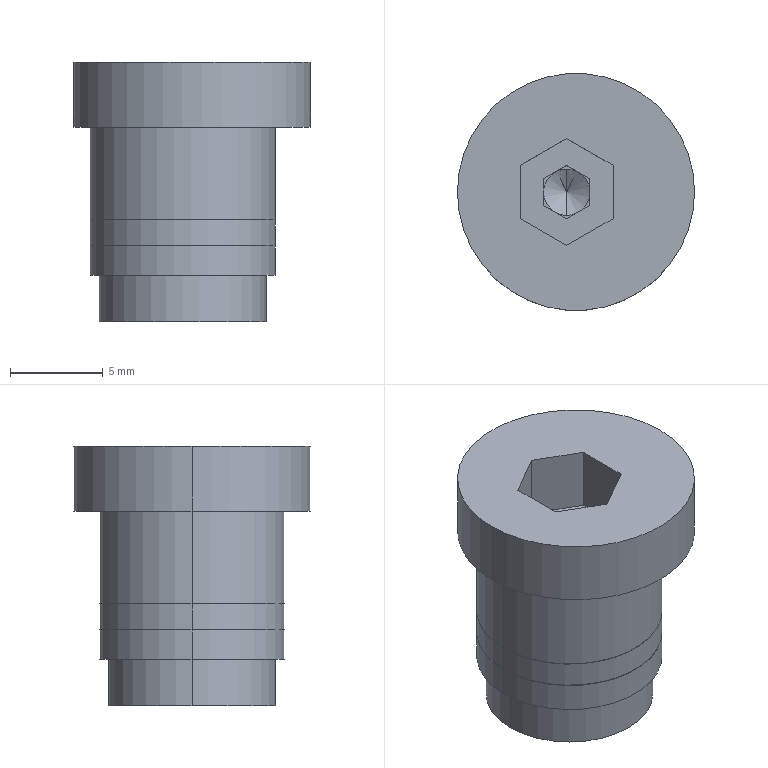Part | STEP file | ASND-0110-偏心销1 | 1 solid | 41 faces | box 12.8 x 12.8 x 14 mm | volume 1139 mm3 | plane 25 | cylinder 10 | cone 6 | commonest cylinder face diameters 10 x6 9 x2 12.8 x2